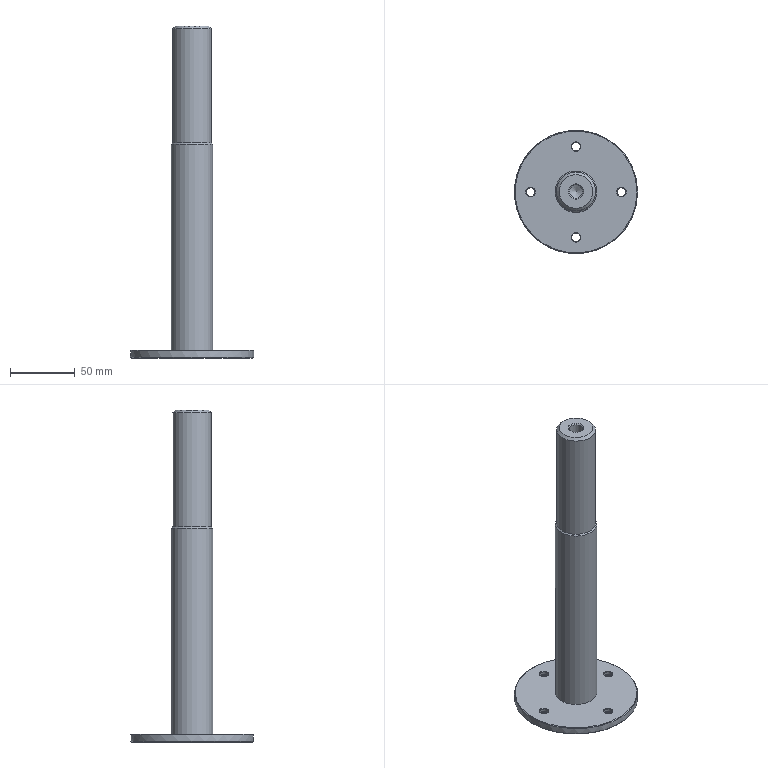Part | NX | features DATUM_CSYS 5, HOLE PACKAGE 5, CSUNK_HOLE 4, EXTRACT_DATUM_AXIS 4, EXTRACT_FACE 4, SKETCH 4, CHAMFER 3, Instance Feature 3, CYLINDER 2, SYMBOLIC_THREAD 2, EXTRUDE 1, Pattern Feature 1, SIMPLE HOLE 1 | 2 solids | 26 faces | box 95 x 95 x 256 mm | volume 230884 mm3 | cone 14 | cylinder 8 | plane 4 | commonest cylinder face diameters 6.6 x4 10.3 x1 30 x1 32 x1 95 x1
STEP:
#1=CARTESIAN_POINT('',(16.,0.,6.));
#2=VERTEX_POINT('',#1);
#3=CARTESIAN_POINT('',(0.,0.,6.));
#4=DIRECTION('',(0.,0.,1.));
#5=DIRECTION('',(1.,0.,0.));
#6=AXIS2_PLACEMENT_3D('',#3,#4,#5);
#7=CIRCLE('',#6,16.);
#8=EDGE_CURVE('',#2,#2,#7,.T.);
#9=ORIENTED_EDGE('',*,*,#8,.F.);
#10=EDGE_LOOP('',(#9));
#11=FACE_BOUND('',#10,.T.);
#12=CARTESIAN_POINT('',(0.,0.,6.));
#13=DIRECTION('',(0.,0.,-1.));
#14=DIRECTION('',(-1.,0.,0.));
#15=AXIS2_PLACEMENT_3D('',#12,#13,#14);
#16=PLANE('',#15);
#17=ADVANCED_FACE('',(#11),#16,.T.);
#18=CARTESIAN_POINT('',(16.,0.,165.));
#19=VERTEX_POINT('',#18);
#20=CARTESIAN_POINT('',(0.,0.,165.));
#21=DIRECTION('',(0.,0.,1.));
#22=DIRECTION('',(1.,0.,0.));
#23=AXIS2_PLACEMENT_3D('',#20,#21,#22);
#24=CIRCLE('',#23,16.);
#25=EDGE_CURVE('',#19,#19,#24,.F.);
#26=ORIENTED_EDGE('',*,*,#25,.T.);
#27=EDGE_LOOP('',(#26));
#28=FACE_BOUND('',#27,.T.);
#29=ORIENTED_EDGE('',*,*,#8,.T.);
#30=EDGE_LOOP('',(#29));
#31=FACE_BOUND('',#30,.T.);
#32=CARTESIAN_POINT('',(0.,0.,6.));
#33=DIRECTION('',(0.,0.,1.));
#34=DIRECTION('',(1.,0.,0.));
#35=AXIS2_PLACEMENT_3D('',#32,#33,#34);
#36=CYLINDRICAL_SURFACE('',#35,16.);
#37=ADVANCED_FACE('',(#28,#31),#36,.T.);
#38=CARTESIAN_POINT('',(15.,0.,254.));
#39=VERTEX_POINT('',#38);
#40=CARTESIAN_POINT('',(0.,0.,254.));
#41=DIRECTION('',(0.,0.,1.));
#42=DIRECTION('',(1.,0.,0.));
#43=AXIS2_PLACEMENT_3D('',#40,#41,#42);
#44=CIRCLE('',#43,15.);
#45=EDGE_CURVE('',#39,#39,#44,.F.);
#46=ORIENTED_EDGE('',*,*,#45,.T.);
#47=EDGE_LOOP('',(#46));
#48=FACE_BOUND('',#47,.T.);
#49=CARTESIAN_POINT('',(-15.,0.,166.));
#50=VERTEX_POINT('',#49);
#51=CARTESIAN_POINT('',(0.,0.,166.));
#52=DIRECTION('',(0.,0.,-1.));
#53=DIRECTION('',(-1.,0.,0.));
#54=AXIS2_PLACEMENT_3D('',#51,#52,#53);
#55=CIRCLE('',#54,15.);
#56=EDGE_CURVE('',#50,#50,#55,.T.);
#57=ORIENTED_EDGE('',*,*,#56,.F.);
#58=EDGE_LOOP('',(#57));
#59=FACE_BOUND('',#58,.T.);
#60=CARTESIAN_POINT('',(0.,0.,256.));
#61=DIRECTION('',(0.,0.,-1.));
#62=DIRECTION('',(-1.,0.,0.));
#63=AXIS2_PLACEMENT_3D('',#60,#61,#62);
#64=CYLINDRICAL_SURFACE('',#63,15.);
#65=ADVANCED_FACE('',(#48,#59),#64,.T.);
#66=CARTESIAN_POINT('',(6.,0.,256.));
#67=VERTEX_POINT('',#66);
#68=CARTESIAN_POINT('',(0.,0.,256.));
#69=DIRECTION('',(0.,0.,1.));
#70=DIRECTION('',(1.,0.,0.));
#71=AXIS2_PLACEMENT_3D('',#68,#69,#70);
#72=CIRCLE('',#71,6.);
#73=EDGE_CURVE('',#67,#67,#72,.F.);
#74=ORIENTED_EDGE('',*,*,#73,.T.);
#75=EDGE_LOOP('',(#74));
#76=FACE_BOUND('',#75,.T.);
#77=CARTESIAN_POINT('',(13.,0.,256.));
#78=VERTEX_POINT('',#77);
#79=CARTESIAN_POINT('',(0.,0.,256.));
#80=DIRECTION('',(0.,0.,1.));
#81=DIRECTION('',(1.,0.,0.));
#82=AXIS2_PLACEMENT_3D('',#79,#80,#81);
#83=CIRCLE('',#82,13.);
#84=EDGE_CURVE('',#78,#78,#83,.T.);
#85=ORIENTED_EDGE('',*,*,#84,.T.);
#86=EDGE_LOOP('',(#85));
#87=FACE_BOUND('',#86,.T.);
#88=CARTESIAN_POINT('',(0.,0.,256.));
#89=DIRECTION('',(0.,0.,1.));
#90=DIRECTION('',(1.,0.,0.));
#91=AXIS2_PLACEMENT_3D('',#88,#89,#90);
#92=PLANE('',#91);
#93=ADVANCED_FACE('',(#76,#87),#92,.T.);
#94=ORIENTED_EDGE('',*,*,#25,.F.);
#95=EDGE_LOOP('',(#94));
#96=FACE_BOUND('',#95,.T.);
#97=ORIENTED_EDGE('',*,*,#56,.T.);
#98=EDGE_LOOP('',(#97));
#99=FACE_BOUND('',#98,.T.);
#100=CARTESIAN_POINT('',(0.,0.,166.));
#101=DIRECTION('',(0.,0.,-1.));
#102=DIRECTION('',(-1.,0.,0.));
#103=AXIS2_PLACEMENT_3D('',#100,#101,#102);
#104=CONICAL_SURFACE('',#103,15.,0.7854);
#105=ADVANCED_FACE('',(#96,#99),#104,.T.);
#106=ORIENTED_EDGE('',*,*,#45,.F.);
#107=EDGE_LOOP('',(#106));
#108=FACE_BOUND('',#107,.T.);
#109=ORIENTED_EDGE('',*,*,#84,.F.);
#110=EDGE_LOOP('',(#109));
#111=FACE_BOUND('',#110,.T.);
#112=CARTESIAN_POINT('',(0.,0.,256.));
#113=DIRECTION('',(0.,0.,-1.));
#114=DIRECTION('',(-1.,0.,0.));
#115=AXIS2_PLACEMENT_3D('',#112,#113,#114);
#116=CONICAL_SURFACE('',#115,13.,0.7854);
#117=ADVANCED_FACE('',(#108,#111),#116,.T.);
#118=CARTESIAN_POINT('',(-5.15,0.,232.));
#119=VERTEX_POINT('',#118);
#120=CARTESIAN_POINT('',(0.,0.,232.));
#121=DIRECTION('',(0.,0.,-1.));
#122=DIRECTION('',(-1.,0.,0.));
#123=AXIS2_PLACEMENT_3D('',#120,#121,#122);
#124=CIRCLE('',#123,5.15);
#125=EDGE_CURVE('',#119,#119,#124,.F.);
#126=ORIENTED_EDGE('',*,*,#125,.T.);
#127=EDGE_LOOP('',(#126));
#128=FACE_BOUND('',#127,.T.);
#129=CARTESIAN_POINT('',(0.,0.,228.906));
#130=VERTEX_POINT('',#129);
#131=VERTEX_LOOP('',#130);
#132=FACE_BOUND('',#131,.T.);
#133=CARTESIAN_POINT('',(0.,0.,232.));
#134=DIRECTION('',(0.,0.,1.));
#135=DIRECTION('',(1.,0.,0.));
#136=AXIS2_PLACEMENT_3D('',#133,#134,#135);
#137=CONICAL_SURFACE('',#136,5.15,1.03);
#138=ADVANCED_FACE('',(#128,#132),#137,.F.);
#139=CARTESIAN_POINT('',(5.15,0.,255.15));
#140=VERTEX_POINT('',#139);
#141=CARTESIAN_POINT('',(0.,0.,255.15));
#142=DIRECTION('',(0.,0.,1.));
#143=DIRECTION('',(1.,0.,0.));
#144=AXIS2_PLACEMENT_3D('',#141,#142,#143);
#145=CIRCLE('',#144,5.15);
#146=EDGE_CURVE('',#140,#140,#145,.T.);
#147=ORIENTED_EDGE('',*,*,#146,.T.);
#148=EDGE_LOOP('',(#147));
#149=FACE_BOUND('',#148,.T.);
#150=ORIENTED_EDGE('',*,*,#125,.F.);
#151=EDGE_LOOP('',(#150));
#152=FACE_BOUND('',#151,.T.);
#153=CARTESIAN_POINT('',(0.,0.,256.));
#154=DIRECTION('',(0.,0.,-1.));
#155=DIRECTION('',(-1.,0.,0.));
#156=AXIS2_PLACEMENT_3D('',#153,#154,#155);
#157=CYLINDRICAL_SURFACE('',#156,5.15);
#158=ADVANCED_FACE('',(#149,#152),#157,.F.);
#159=ORIENTED_EDGE('',*,*,#146,.F.);
#160=EDGE_LOOP('',(#159));
#161=FACE_BOUND('',#160,.T.);
#162=ORIENTED_EDGE('',*,*,#73,.F.);
#163=EDGE_LOOP('',(#162));
#164=FACE_BOUND('',#163,.T.);
#165=CARTESIAN_POINT('',(0.,0.,256.));
#166=DIRECTION('',(0.,0.,1.));
#167=DIRECTION('',(1.,0.,0.));
#168=AXIS2_PLACEMENT_3D('',#165,#166,#167);
#169=CONICAL_SURFACE('',#168,6.,0.7854);
#170=ADVANCED_FACE('',(#161,#164),#169,.F.);
#171=CLOSED_SHELL('',(#17,#37,#65,#93,#105,#117,#138,#158,#170));
#172=MANIFOLD_SOLID_BREP('',#171);
#173=CARTESIAN_POINT('',(3.7,35.,6.));
#174=VERTEX_POINT('',#173);
#175=CARTESIAN_POINT('',(0.,35.,6.));
#176=DIRECTION('',(0.,0.,1.));
#177=DIRECTION('',(1.,0.,0.));
#178=AXIS2_PLACEMENT_3D('',#175,#176,#177);
#179=CIRCLE('',#178,3.7);
#180=EDGE_CURVE('',#174,#174,#179,.F.);
#181=ORIENTED_EDGE('',*,*,#180,.T.);
#182=EDGE_LOOP('',(#181));
#183=FACE_BOUND('',#182,.T.);
#184=CARTESIAN_POINT('',(-31.3,0.,6.));
#185=VERTEX_POINT('',#184);
#186=CARTESIAN_POINT('',(-35.,0.,6.));
#187=DIRECTION('',(0.,0.,1.));
#188=DIRECTION('',(1.,0.,0.));
#189=AXIS2_PLACEMENT_3D('',#186,#187,#188);
#190=CIRCLE('',#189,3.7);
#191=EDGE_CURVE('',#185,#185,#190,.F.);
#192=ORIENTED_EDGE('',*,*,#191,.T.);
#193=EDGE_LOOP('',(#192));
#194=FACE_BOUND('',#193,.T.);
#195=CARTESIAN_POINT('',(3.7,-35.,6.));
#196=VERTEX_POINT('',#195);
#197=CARTESIAN_POINT('',(0.,-35.,6.));
#198=DIRECTION('',(0.,0.,1.));
#199=DIRECTION('',(1.,0.,0.));
#200=AXIS2_PLACEMENT_3D('',#197,#198,#199);
#201=CIRCLE('',#200,3.7);
#202=EDGE_CURVE('',#196,#196,#201,.F.);
#203=ORIENTED_EDGE('',*,*,#202,.T.);
#204=EDGE_LOOP('',(#203));
#205=FACE_BOUND('',#204,.T.);
#206=CARTESIAN_POINT('',(38.7,0.,6.));
#207=VERTEX_POINT('',#206);
#208=CARTESIAN_POINT('',(35.,0.,6.));
#209=DIRECTION('',(0.,0.,1.));
#210=DIRECTION('',(1.,0.,0.));
#211=AXIS2_PLACEMENT_3D('',#208,#209,#210);
#212=CIRCLE('',#211,3.7);
#213=EDGE_CURVE('',#207,#207,#212,.F.);
#214=ORIENTED_EDGE('',*,*,#213,.T.);
#215=EDGE_LOOP('',(#214));
#216=FACE_BOUND('',#215,.T.);
#217=CARTESIAN_POINT('',(47.,0.,6.));
#218=VERTEX_POINT('',#217);
#219=CARTESIAN_POINT('',(0.,0.,6.));
#220=DIRECTION('',(0.,0.,1.));
#221=DIRECTION('',(1.,0.,0.));
#222=AXIS2_PLACEMENT_3D('',#219,#220,#221);
#223=CIRCLE('',#222,47.);
#224=EDGE_CURVE('',#218,#218,#223,.T.);
#225=ORIENTED_EDGE('',*,*,#224,.T.);
#226=EDGE_LOOP('',(#225));
#227=FACE_BOUND('',#226,.T.);
#228=CARTESIAN_POINT('',(0.,0.,6.));
#229=DIRECTION('',(0.,0.,1.));
#230=DIRECTION('',(1.,0.,0.));
#231=AXIS2_PLACEMENT_3D('',#228,#229,#230);
#232=PLANE('',#231);
#233=ADVANCED_FACE('',(#183,#194,#205,#216,#227),#232,.T.);
#234=CARTESIAN_POINT('',(6.855,35.,0.));
#235=VERTEX_POINT('',#234);
#236=CARTESIAN_POINT('',(0.,35.,0.));
#237=DIRECTION('',(0.,0.,1.));
#238=DIRECTION('',(1.,0.,0.));
#239=AXIS2_PLACEMENT_3D('',#236,#237,#238);
#240=CIRCLE('',#239,6.855);
#241=EDGE_CURVE('',#235,#235,#240,.T.);
#242=ORIENTED_EDGE('',*,*,#241,.T.);
#243=EDGE_LOOP('',(#242));
#244=FACE_BOUND('',#243,.T.);
#245=CARTESIAN_POINT('',(-28.145,0.,0.));
#246=VERTEX_POINT('',#245);
#247=CARTESIAN_POINT('',(-35.,0.,0.));
#248=DIRECTION('',(0.,0.,1.));
#249=DIRECTION('',(1.,0.,0.));
#250=AXIS2_PLACEMENT_3D('',#247,#248,#249);
#251=CIRCLE('',#250,6.855);
#252=EDGE_CURVE('',#246,#246,#251,.T.);
#253=ORIENTED_EDGE('',*,*,#252,.T.);
#254=EDGE_LOOP('',(#253));
#255=FACE_BOUND('',#254,.T.);
#256=CARTESIAN_POINT('',(6.855,-35.,0.));
#257=VERTEX_POINT('',#256);
#258=CARTESIAN_POINT('',(0.,-35.,0.));
#259=DIRECTION('',(0.,0.,1.));
#260=DIRECTION('',(1.,0.,0.));
#261=AXIS2_PLACEMENT_3D('',#258,#259,#260);
#262=CIRCLE('',#261,6.855);
#263=EDGE_CURVE('',#257,#257,#262,.T.);
#264=ORIENTED_EDGE('',*,*,#263,.T.);
#265=EDGE_LOOP('',(#264));
#266=FACE_BOUND('',#265,.T.);
#267=CARTESIAN_POINT('',(41.855,0.,0.));
#268=VERTEX_POINT('',#267);
#269=CARTESIAN_POINT('',(35.,0.,0.));
#270=DIRECTION('',(0.,0.,1.));
#271=DIRECTION('',(1.,0.,0.));
#272=AXIS2_PLACEMENT_3D('',#269,#270,#271);
#273=CIRCLE('',#272,6.855);
#274=EDGE_CURVE('',#268,#268,#273,.T.);
#275=ORIENTED_EDGE('',*,*,#274,.T.);
#276=EDGE_LOOP('',(#275));
#277=FACE_BOUND('',#276,.T.);
#278=CARTESIAN_POINT('',(-47.,0.,0.));
#279=VERTEX_POINT('',#278);
#280=CARTESIAN_POINT('',(0.,0.,0.));
#281=DIRECTION('',(0.,0.,-1.));
#282=DIRECTION('',(-1.,0.,0.));
#283=AXIS2_PLACEMENT_3D('',#280,#281,#282);
#284=CIRCLE('',#283,47.);
#285=EDGE_CURVE('',#279,#279,#284,.T.);
#286=ORIENTED_EDGE('',*,*,#285,.T.);
#287=EDGE_LOOP('',(#286));
#288=FACE_BOUND('',#287,.T.);
#289=CARTESIAN_POINT('',(0.,0.,0.));
#290=DIRECTION('',(0.,0.,-1.));
#291=DIRECTION('',(-1.,0.,0.));
#292=AXIS2_PLACEMENT_3D('',#289,#290,#291);
#293=PLANE('',#292);
#294=ADVANCED_FACE('',(#244,#255,#266,#277,#288),#293,.T.);
#295=CARTESIAN_POINT('',(-47.5,0.,0.5));
#296=VERTEX_POINT('',#295);
#297=CARTESIAN_POINT('',(0.,0.,0.5));
#298=DIRECTION('',(0.,0.,-1.));
#299=DIRECTION('',(-1.,0.,0.));
#300=AXIS2_PLACEMENT_3D('',#297,#298,#299);
#301=CIRCLE('',#300,47.5);
#302=EDGE_CURVE('',#296,#296,#301,.F.);
#303=ORIENTED_EDGE('',*,*,#302,.T.);
#304=EDGE_LOOP('',(#303));
#305=FACE_BOUND('',#304,.T.);
#306=CARTESIAN_POINT('',(47.5,0.,5.5));
#307=VERTEX_POINT('',#306);
#308=CARTESIAN_POINT('',(0.,0.,5.5));
#309=DIRECTION('',(0.,0.,1.));
#310=DIRECTION('',(1.,0.,0.));
#311=AXIS2_PLACEMENT_3D('',#308,#309,#310);
#312=CIRCLE('',#311,47.5);
#313=EDGE_CURVE('',#307,#307,#312,.F.);
#314=ORIENTED_EDGE('',*,*,#313,.T.);
#315=EDGE_LOOP('',(#314));
#316=FACE_BOUND('',#315,.T.);
#317=CARTESIAN_POINT('',(0.,0.,0.));
#318=DIRECTION('',(0.,0.,1.));
#319=DIRECTION('',(1.,0.,0.));
#320=AXIS2_PLACEMENT_3D('',#317,#318,#319);
#321=CYLINDRICAL_SURFACE('',#320,47.5);
#322=ADVANCED_FACE('',(#305,#316),#321,.T.);
#323=ORIENTED_EDGE('',*,*,#285,.F.);
#324=EDGE_LOOP('',(#323));
#325=FACE_BOUND('',#324,.T.);
#326=ORIENTED_EDGE('',*,*,#302,.F.);
#327=EDGE_LOOP('',(#326));
#328=FACE_BOUND('',#327,.T.);
#329=CARTESIAN_POINT('',(0.,0.,0.5));
#330=DIRECTION('',(0.,0.,1.));
#331=DIRECTION('',(1.,0.,0.));
#332=AXIS2_PLACEMENT_3D('',#329,#330,#331);
#333=CONICAL_SURFACE('',#332,47.5,0.7854);
#334=ADVANCED_FACE('',(#325,#328),#333,.T.);
#335=ORIENTED_EDGE('',*,*,#224,.F.);
#336=EDGE_LOOP('',(#335));
#337=FACE_BOUND('',#336,.T.);
#338=ORIENTED_EDGE('',*,*,#313,.F.);
#339=EDGE_LOOP('',(#338));
#340=FACE_BOUND('',#339,.T.);
#341=CARTESIAN_POINT('',(0.,0.,5.5));
#342=DIRECTION('',(0.,0.,-1.));
#343=DIRECTION('',(-1.,0.,0.));
#344=AXIS2_PLACEMENT_3D('',#341,#342,#343);
#345=CONICAL_SURFACE('',#344,47.5,0.7854);
#346=ADVANCED_FACE('',(#337,#340),#345,.T.);
#347=CARTESIAN_POINT('',(38.3,0.,5.6));
#348=VERTEX_POINT('',#347);
#349=CARTESIAN_POINT('',(35.,0.,5.6));
#350=DIRECTION('',(0.,0.,1.));
#351=DIRECTION('',(1.,0.,0.));
#352=AXIS2_PLACEMENT_3D('',#349,#350,#351);
#353=CIRCLE('',#352,3.3);
#354=EDGE_CURVE('',#348,#348,#353,.T.);
#355=ORIENTED_EDGE('',*,*,#354,.T.);
#356=EDGE_LOOP('',(#355));
#357=FACE_BOUND('',#356,.T.);
#358=CARTESIAN_POINT('',(38.3,0.,3.555));
#359=VERTEX_POINT('',#358);
#360=CARTESIAN_POINT('',(35.,0.,3.555));
#361=DIRECTION('',(0.,0.,1.));
#362=DIRECTION('',(1.,0.,0.));
#363=AXIS2_PLACEMENT_3D('',#360,#361,#362);
#364=CIRCLE('',#363,3.3);
#365=EDGE_CURVE('',#359,#359,#364,.F.);
#366=ORIENTED_EDGE('',*,*,#365,.T.);
#367=EDGE_LOOP('',(#366));
#368=FACE_BOUND('',#367,.T.);
#369=CARTESIAN_POINT('',(35.,0.,50.));
#370=DIRECTION('',(0.,0.,1.));
#371=DIRECTION('',(1.,0.,0.));
#372=AXIS2_PLACEMENT_3D('',#369,#370,#371);
#373=CYLINDRICAL_SURFACE('',#372,3.3);
#374=ADVANCED_FACE('',(#357,#368),#373,.F.);
#375=ORIENTED_EDGE('',*,*,#365,.F.);
#376=EDGE_LOOP('',(#375));
#377=FACE_BOUND('',#376,.T.);
#378=ORIENTED_EDGE('',*,*,#274,.F.);
#379=EDGE_LOOP('',(#378));
#380=FACE_BOUND('',#379,.T.);
#381=CARTESIAN_POINT('',(35.,0.,0.));
#382=DIRECTION('',(0.,0.,-1.));
#383=DIRECTION('',(-1.,0.,0.));
#384=AXIS2_PLACEMENT_3D('',#381,#382,#383);
#385=CONICAL_SURFACE('',#384,6.855,0.7854);
#386=ADVANCED_FACE('',(#377,#380),#385,.F.);
#387=ORIENTED_EDGE('',*,*,#213,.F.);
#388=EDGE_LOOP('',(#387));
#389=FACE_BOUND('',#388,.T.);
#390=ORIENTED_EDGE('',*,*,#354,.F.);
#391=EDGE_LOOP('',(#390));
#392=FACE_BOUND('',#391,.T.);
#393=CARTESIAN_POINT('',(35.,0.,5.6));
#394=DIRECTION('',(0.,0.,1.));
#395=DIRECTION('',(1.,0.,0.));
#396=AXIS2_PLACEMENT_3D('',#393,#394,#395);
#397=CONICAL_SURFACE('',#396,3.3,0.7854);
#398=ADVANCED_FACE('',(#389,#392),#397,.F.);
#399=CARTESIAN_POINT('',(3.3,-35.,5.6));
#400=VERTEX_POINT('',#399);
#401=CARTESIAN_POINT('',(0.,-35.,5.6));
#402=DIRECTION('',(0.,0.,1.));
#403=DIRECTION('',(1.,0.,0.));
#404=AXIS2_PLACEMENT_3D('',#401,#402,#403);
#405=CIRCLE('',#404,3.3);
#406=EDGE_CURVE('',#400,#400,#405,.T.);
#407=ORIENTED_EDGE('',*,*,#406,.T.);
#408=EDGE_LOOP('',(#407));
#409=FACE_BOUND('',#408,.T.);
#410=CARTESIAN_POINT('',(3.3,-35.,3.555));
#411=VERTEX_POINT('',#410);
#412=CARTESIAN_POINT('',(0.,-35.,3.555));
#413=DIRECTION('',(0.,0.,1.));
#414=DIRECTION('',(1.,0.,0.));
#415=AXIS2_PLACEMENT_3D('',#412,#413,#414);
#416=CIRCLE('',#415,3.3);
#417=EDGE_CURVE('',#411,#411,#416,.F.);
#418=ORIENTED_EDGE('',*,*,#417,.T.);
#419=EDGE_LOOP('',(#418));
#420=FACE_BOUND('',#419,.T.);
#421=CARTESIAN_POINT('',(0.,-35.,50.));
#422=DIRECTION('',(0.,0.,1.));
#423=DIRECTION('',(1.,0.,0.));
#424=AXIS2_PLACEMENT_3D('',#421,#422,#423);
#425=CYLINDRICAL_SURFACE('',#424,3.3);
#426=ADVANCED_FACE('',(#409,#420),#425,.F.);
#427=ORIENTED_EDGE('',*,*,#417,.F.);
#428=EDGE_LOOP('',(#427));
#429=FACE_BOUND('',#428,.T.);
#430=ORIENTED_EDGE('',*,*,#263,.F.);
#431=EDGE_LOOP('',(#430));
#432=FACE_BOUND('',#431,.T.);
#433=CARTESIAN_POINT('',(0.,-35.,0.));
#434=DIRECTION('',(0.,0.,-1.));
#435=DIRECTION('',(-1.,0.,0.));
#436=AXIS2_PLACEMENT_3D('',#433,#434,#435);
#437=CONICAL_SURFACE('',#436,6.855,0.7854);
#438=ADVANCED_FACE('',(#429,#432),#437,.F.);
#439=ORIENTED_EDGE('',*,*,#202,.F.);
#440=EDGE_LOOP('',(#439));
#441=FACE_BOUND('',#440,.T.);
#442=ORIENTED_EDGE('',*,*,#406,.F.);
#443=EDGE_LOOP('',(#442));
#444=FACE_BOUND('',#443,.T.);
#445=CARTESIAN_POINT('',(0.,-35.,5.6));
#446=DIRECTION('',(0.,0.,1.));
#447=DIRECTION('',(1.,0.,0.));
#448=AXIS2_PLACEMENT_3D('',#445,#446,#447);
#449=CONICAL_SURFACE('',#448,3.3,0.7854);
#450=ADVANCED_FACE('',(#441,#444),#449,.F.);
#451=CARTESIAN_POINT('',(-31.7,0.,5.6));
#452=VERTEX_POINT('',#451);
#453=CARTESIAN_POINT('',(-35.,0.,5.6));
#454=DIRECTION('',(0.,0.,1.));
#455=DIRECTION('',(1.,0.,0.));
#456=AXIS2_PLACEMENT_3D('',#453,#454,#455);
#457=CIRCLE('',#456,3.3);
#458=EDGE_CURVE('',#452,#452,#457,.T.);
#459=ORIENTED_EDGE('',*,*,#458,.T.);
#460=EDGE_LOOP('',(#459));
#461=FACE_BOUND('',#460,.T.);
#462=CARTESIAN_POINT('',(-31.7,0.,3.555));
#463=VERTEX_POINT('',#462);
#464=CARTESIAN_POINT('',(-35.,0.,3.555));
#465=DIRECTION('',(0.,0.,1.));
#466=DIRECTION('',(1.,0.,0.));
#467=AXIS2_PLACEMENT_3D('',#464,#465,#466);
#468=CIRCLE('',#467,3.3);
#469=EDGE_CURVE('',#463,#463,#468,.F.);
#470=ORIENTED_EDGE('',*,*,#469,.T.);
#471=EDGE_LOOP('',(#470));
#472=FACE_BOUND('',#471,.T.);
#473=CARTESIAN_POINT('',(-35.,0.,50.));
#474=DIRECTION('',(0.,0.,1.));
#475=DIRECTION('',(1.,0.,0.));
#476=AXIS2_PLACEMENT_3D('',#473,#474,#475);
#477=CYLINDRICAL_SURFACE('',#476,3.3);
#478=ADVANCED_FACE('',(#461,#472),#477,.F.);
#479=ORIENTED_EDGE('',*,*,#469,.F.);
#480=EDGE_LOOP('',(#479));
#481=FACE_BOUND('',#480,.T.);
#482=ORIENTED_EDGE('',*,*,#252,.F.);
#483=EDGE_LOOP('',(#482));
#484=FACE_BOUND('',#483,.T.);
#485=CARTESIAN_POINT('',(-35.,0.,0.));
#486=DIRECTION('',(0.,0.,-1.));
#487=DIRECTION('',(-1.,0.,0.));
#488=AXIS2_PLACEMENT_3D('',#485,#486,#487);
#489=CONICAL_SURFACE('',#488,6.855,0.7854);
#490=ADVANCED_FACE('',(#481,#484),#489,.F.);
#491=ORIENTED_EDGE('',*,*,#191,.F.);
#492=EDGE_LOOP('',(#491));
#493=FACE_BOUND('',#492,.T.);
#494=ORIENTED_EDGE('',*,*,#458,.F.);
#495=EDGE_LOOP('',(#494));
#496=FACE_BOUND('',#495,.T.);
#497=CARTESIAN_POINT('',(-35.,0.,5.6));
#498=DIRECTION('',(0.,0.,1.));
#499=DIRECTION('',(1.,0.,0.));
#500=AXIS2_PLACEMENT_3D('',#497,#498,#499);
#501=CONICAL_SURFACE('',#500,3.3,0.7854);
#502=ADVANCED_FACE('',(#493,#496),#501,.F.);
#503=CARTESIAN_POINT('',(3.3,35.,5.6));
#504=VERTEX_POINT('',#503);
#505=CARTESIAN_POINT('',(0.,35.,5.6));
#506=DIRECTION('',(0.,0.,1.));
#507=DIRECTION('',(1.,0.,0.));
#508=AXIS2_PLACEMENT_3D('',#505,#506,#507);
#509=CIRCLE('',#508,3.3);
#510=EDGE_CURVE('',#504,#504,#509,.T.);
#511=ORIENTED_EDGE('',*,*,#510,.T.);
#512=EDGE_LOOP('',(#511));
#513=FACE_BOUND('',#512,.T.);
#514=CARTESIAN_POINT('',(3.3,35.,3.555));
#515=VERTEX_POINT('',#514);
#516=CARTESIAN_POINT('',(0.,35.,3.555));
#517=DIRECTION('',(0.,0.,1.));
#518=DIRECTION('',(1.,0.,0.));
#519=AXIS2_PLACEMENT_3D('',#516,#517,#518);
#520=CIRCLE('',#519,3.3);
#521=EDGE_CURVE('',#515,#515,#520,.F.);
#522=ORIENTED_EDGE('',*,*,#521,.T.);
#523=EDGE_LOOP('',(#522));
#524=FACE_BOUND('',#523,.T.);
#525=CARTESIAN_POINT('',(0.,35.,50.));
#526=DIRECTION('',(0.,0.,1.));
#527=DIRECTION('',(1.,0.,0.));
#528=AXIS2_PLACEMENT_3D('',#525,#526,#527);
#529=CYLINDRICAL_SURFACE('',#528,3.3);
#530=ADVANCED_FACE('',(#513,#524),#529,.F.);
#531=ORIENTED_EDGE('',*,*,#521,.F.);
#532=EDGE_LOOP('',(#531));
#533=FACE_BOUND('',#532,.T.);
#534=ORIENTED_EDGE('',*,*,#241,.F.);
#535=EDGE_LOOP('',(#534));
#536=FACE_BOUND('',#535,.T.);
#537=CARTESIAN_POINT('',(0.,35.,0.));
#538=DIRECTION('',(0.,0.,-1.));
#539=DIRECTION('',(-1.,0.,0.));
#540=AXIS2_PLACEMENT_3D('',#537,#538,#539);
#541=CONICAL_SURFACE('',#540,6.855,0.7854);
#542=ADVANCED_FACE('',(#533,#536),#541,.F.);
#543=ORIENTED_EDGE('',*,*,#180,.F.);
#544=EDGE_LOOP('',(#543));
#545=FACE_BOUND('',#544,.T.);
#546=ORIENTED_EDGE('',*,*,#510,.F.);
#547=EDGE_LOOP('',(#546));
#548=FACE_BOUND('',#547,.T.);
#549=CARTESIAN_POINT('',(0.,35.,5.6));
#550=DIRECTION('',(0.,0.,1.));
#551=DIRECTION('',(1.,0.,0.));
#552=AXIS2_PLACEMENT_3D('',#549,#550,#551);
#553=CONICAL_SURFACE('',#552,3.3,0.7854);
#554=ADVANCED_FACE('',(#545,#548),#553,.F.);
#555=CLOSED_SHELL('',(#233,#294,#322,#334,#346,#374,#386,#398,#426,#438,#450,#478,#490,#502,#530,#542,#554));
#556=MANIFOLD_SOLID_BREP('',#555);
#557=(LENGTH_UNIT()NAMED_UNIT(*)SI_UNIT(.MILLI.,.METRE.));
#558=UNCERTAINTY_MEASURE_WITH_UNIT(LENGTH_MEASURE(0.00001),#557,'','');
#559=(NAMED_UNIT(*)PLANE_ANGLE_UNIT()SI_UNIT($,.RADIAN.));
#560=(NAMED_UNIT(*)SI_UNIT($,.STERADIAN.)SOLID_ANGLE_UNIT());
#561=(GEOMETRIC_REPRESENTATION_CONTEXT(3)GLOBAL_UNCERTAINTY_ASSIGNED_CONTEXT((#558))GLOBAL_UNIT_ASSIGNED_CONTEXT((#557,#559,#560))REPRESENTATION_CONTEXT('',''));
#562=ADVANCED_BREP_SHAPE_REPRESENTATION('',(#172,#556),#561);